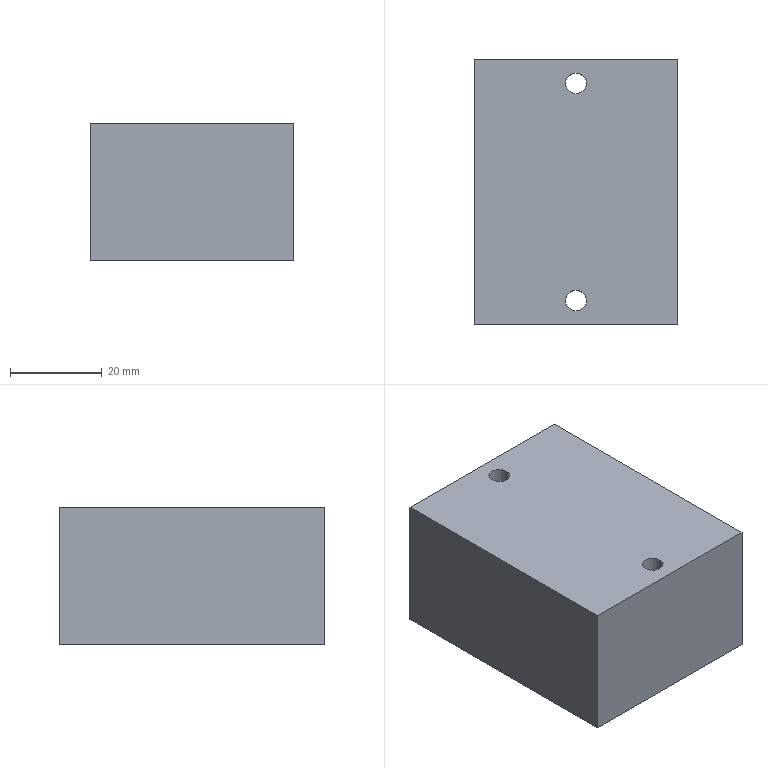Part | SolidWorks | features Extrusion 1 | 1 solid | 10 faces | box 44.5 x 58 x 30 mm | volume 76476 mm3 | plane 6 | cylinder 4 | commonest cylinder face diameters 4.5 x4
STEP:
#1=CARTESIAN_POINT('',(-2.25,-23.7,30.));
#2=VERTEX_POINT('',#1);
#3=CARTESIAN_POINT('',(2.25,-23.7,30.));
#4=VERTEX_POINT('',#3);
#5=CARTESIAN_POINT('',(0.,-23.7,30.));
#6=DIRECTION('',(0.,0.,1.));
#7=DIRECTION('',(1.,0.,0.));
#8=AXIS2_PLACEMENT_3D('',#5,#6,#7);
#9=CIRCLE('',#8,2.25);
#10=EDGE_CURVE('',#2,#4,#9,.T.);
#11=ORIENTED_EDGE('',*,*,#10,.T.);
#12=CARTESIAN_POINT('',(2.25,-23.7,0.));
#13=VERTEX_POINT('',#12);
#14=CARTESIAN_POINT('',(2.25,-23.7,30.));
#15=DIRECTION('',(0.,0.,-1.));
#16=VECTOR('',#15,1000.);
#17=LINE('',#14,#16);
#18=EDGE_CURVE('',#4,#13,#17,.T.);
#19=ORIENTED_EDGE('',*,*,#18,.T.);
#20=CARTESIAN_POINT('',(-2.25,-23.7,0.));
#21=VERTEX_POINT('',#20);
#22=CARTESIAN_POINT('',(0.,-23.7,0.));
#23=DIRECTION('',(0.,0.,1.));
#24=DIRECTION('',(1.,0.,0.));
#25=AXIS2_PLACEMENT_3D('',#22,#23,#24);
#26=CIRCLE('',#25,2.25);
#27=EDGE_CURVE('',#21,#13,#26,.T.);
#28=ORIENTED_EDGE('',*,*,#27,.F.);
#29=CARTESIAN_POINT('',(-2.25,-23.7,30.));
#30=DIRECTION('',(0.,0.,-1.));
#31=VECTOR('',#30,1000.);
#32=LINE('',#29,#31);
#33=EDGE_CURVE('',#2,#21,#32,.T.);
#34=ORIENTED_EDGE('',*,*,#33,.F.);
#35=EDGE_LOOP('',(#11,#19,#28,#34));
#36=FACE_OUTER_BOUND('',#35,.T.);
#37=CARTESIAN_POINT('',(0.,-23.7,30.));
#38=DIRECTION('',(0.,0.,-1.));
#39=DIRECTION('',(-1.,0.,0.));
#40=AXIS2_PLACEMENT_3D('',#37,#38,#39);
#41=CYLINDRICAL_SURFACE('',#40,2.25);
#42=ADVANCED_FACE('',(#36),#41,.F.);
#43=CARTESIAN_POINT('',(-2.25,23.7,30.));
#44=VERTEX_POINT('',#43);
#45=CARTESIAN_POINT('',(2.25,23.7,30.));
#46=VERTEX_POINT('',#45);
#47=CARTESIAN_POINT('',(0.,23.7,30.));
#48=DIRECTION('',(0.,0.,1.));
#49=DIRECTION('',(1.,0.,0.));
#50=AXIS2_PLACEMENT_3D('',#47,#48,#49);
#51=CIRCLE('',#50,2.25);
#52=EDGE_CURVE('',#44,#46,#51,.T.);
#53=ORIENTED_EDGE('',*,*,#52,.T.);
#54=CARTESIAN_POINT('',(2.25,23.7,0.));
#55=VERTEX_POINT('',#54);
#56=CARTESIAN_POINT('',(2.25,23.7,30.));
#57=DIRECTION('',(0.,0.,-1.));
#58=VECTOR('',#57,1000.);
#59=LINE('',#56,#58);
#60=EDGE_CURVE('',#46,#55,#59,.T.);
#61=ORIENTED_EDGE('',*,*,#60,.T.);
#62=CARTESIAN_POINT('',(-2.25,23.7,0.));
#63=VERTEX_POINT('',#62);
#64=CARTESIAN_POINT('',(0.,23.7,0.));
#65=DIRECTION('',(0.,0.,1.));
#66=DIRECTION('',(1.,0.,0.));
#67=AXIS2_PLACEMENT_3D('',#64,#65,#66);
#68=CIRCLE('',#67,2.25);
#69=EDGE_CURVE('',#63,#55,#68,.T.);
#70=ORIENTED_EDGE('',*,*,#69,.F.);
#71=CARTESIAN_POINT('',(-2.25,23.7,30.));
#72=DIRECTION('',(0.,0.,-1.));
#73=VECTOR('',#72,1000.);
#74=LINE('',#71,#73);
#75=EDGE_CURVE('',#44,#63,#74,.T.);
#76=ORIENTED_EDGE('',*,*,#75,.F.);
#77=EDGE_LOOP('',(#53,#61,#70,#76));
#78=FACE_OUTER_BOUND('',#77,.T.);
#79=CARTESIAN_POINT('',(0.,23.7,30.));
#80=DIRECTION('',(0.,0.,-1.));
#81=DIRECTION('',(-1.,0.,0.));
#82=AXIS2_PLACEMENT_3D('',#79,#80,#81);
#83=CYLINDRICAL_SURFACE('',#82,2.25);
#84=ADVANCED_FACE('',(#78),#83,.F.);
#85=CARTESIAN_POINT('',(22.25,-29.,30.));
#86=VERTEX_POINT('',#85);
#87=CARTESIAN_POINT('',(22.25,29.,30.));
#88=VERTEX_POINT('',#87);
#89=CARTESIAN_POINT('',(22.25,-29.,30.));
#90=DIRECTION('',(0.,1.,0.));
#91=VECTOR('',#90,1000.);
#92=LINE('',#89,#91);
#93=EDGE_CURVE('',#86,#88,#92,.T.);
#94=ORIENTED_EDGE('',*,*,#93,.T.);
#95=CARTESIAN_POINT('',(-22.25,29.,30.));
#96=VERTEX_POINT('',#95);
#97=CARTESIAN_POINT('',(-22.25,29.,30.));
#98=DIRECTION('',(-1.,0.,0.));
#99=VECTOR('',#98,1000.);
#100=LINE('',#97,#99);
#101=EDGE_CURVE('',#88,#96,#100,.T.);
#102=ORIENTED_EDGE('',*,*,#101,.T.);
#103=CARTESIAN_POINT('',(-22.25,-29.,30.));
#104=VERTEX_POINT('',#103);
#105=CARTESIAN_POINT('',(-22.25,-29.,30.));
#106=DIRECTION('',(0.,-1.,0.));
#107=VECTOR('',#106,1000.);
#108=LINE('',#105,#107);
#109=EDGE_CURVE('',#96,#104,#108,.T.);
#110=ORIENTED_EDGE('',*,*,#109,.T.);
#111=CARTESIAN_POINT('',(-22.25,-29.,30.));
#112=DIRECTION('',(1.,0.,0.));
#113=VECTOR('',#112,1000.);
#114=LINE('',#111,#113);
#115=EDGE_CURVE('',#104,#86,#114,.T.);
#116=ORIENTED_EDGE('',*,*,#115,.T.);
#117=EDGE_LOOP('',(#94,#102,#110,#116));
#118=FACE_OUTER_BOUND('',#117,.T.);
#119=ORIENTED_EDGE('',*,*,#52,.F.);
#120=CARTESIAN_POINT('',(0.,23.7,30.));
#121=DIRECTION('',(0.,0.,1.));
#122=DIRECTION('',(1.,0.,0.));
#123=AXIS2_PLACEMENT_3D('',#120,#121,#122);
#124=CIRCLE('',#123,2.25);
#125=EDGE_CURVE('',#46,#44,#124,.T.);
#126=ORIENTED_EDGE('',*,*,#125,.F.);
#127=EDGE_LOOP('',(#119,#126));
#128=FACE_BOUND('',#127,.T.);
#129=ORIENTED_EDGE('',*,*,#10,.F.);
#130=CARTESIAN_POINT('',(0.,-23.7,30.));
#131=DIRECTION('',(0.,0.,1.));
#132=DIRECTION('',(1.,0.,0.));
#133=AXIS2_PLACEMENT_3D('',#130,#131,#132);
#134=CIRCLE('',#133,2.25);
#135=EDGE_CURVE('',#4,#2,#134,.T.);
#136=ORIENTED_EDGE('',*,*,#135,.F.);
#137=EDGE_LOOP('',(#129,#136));
#138=FACE_BOUND('',#137,.T.);
#139=CARTESIAN_POINT('',(0.,0.,30.));
#140=DIRECTION('',(0.,0.,-1.));
#141=DIRECTION('',(-1.,0.,0.));
#142=AXIS2_PLACEMENT_3D('',#139,#140,#141);
#143=PLANE('',#142);
#144=ADVANCED_FACE('',(#118,#128,#138),#143,.F.);
#145=ORIENTED_EDGE('',*,*,#69,.T.);
#146=CARTESIAN_POINT('',(0.,23.7,0.));
#147=DIRECTION('',(0.,0.,1.));
#148=DIRECTION('',(1.,0.,0.));
#149=AXIS2_PLACEMENT_3D('',#146,#147,#148);
#150=CIRCLE('',#149,2.25);
#151=EDGE_CURVE('',#55,#63,#150,.T.);
#152=ORIENTED_EDGE('',*,*,#151,.T.);
#153=EDGE_LOOP('',(#145,#152));
#154=FACE_BOUND('',#153,.T.);
#155=CARTESIAN_POINT('',(22.25,-29.,0.));
#156=VERTEX_POINT('',#155);
#157=CARTESIAN_POINT('',(22.25,29.,0.));
#158=VERTEX_POINT('',#157);
#159=CARTESIAN_POINT('',(22.25,-29.,0.));
#160=DIRECTION('',(0.,1.,0.));
#161=VECTOR('',#160,1000.);
#162=LINE('',#159,#161);
#163=EDGE_CURVE('',#156,#158,#162,.T.);
#164=ORIENTED_EDGE('',*,*,#163,.F.);
#165=CARTESIAN_POINT('',(-22.25,-29.,0.));
#166=VERTEX_POINT('',#165);
#167=CARTESIAN_POINT('',(-22.25,-29.,0.));
#168=DIRECTION('',(1.,0.,0.));
#169=VECTOR('',#168,1000.);
#170=LINE('',#167,#169);
#171=EDGE_CURVE('',#166,#156,#170,.T.);
#172=ORIENTED_EDGE('',*,*,#171,.F.);
#173=CARTESIAN_POINT('',(-22.25,29.,0.));
#174=VERTEX_POINT('',#173);
#175=CARTESIAN_POINT('',(-22.25,-29.,0.));
#176=DIRECTION('',(0.,-1.,0.));
#177=VECTOR('',#176,1000.);
#178=LINE('',#175,#177);
#179=EDGE_CURVE('',#174,#166,#178,.T.);
#180=ORIENTED_EDGE('',*,*,#179,.F.);
#181=CARTESIAN_POINT('',(-22.25,29.,0.));
#182=DIRECTION('',(-1.,0.,0.));
#183=VECTOR('',#182,1000.);
#184=LINE('',#181,#183);
#185=EDGE_CURVE('',#158,#174,#184,.T.);
#186=ORIENTED_EDGE('',*,*,#185,.F.);
#187=EDGE_LOOP('',(#164,#172,#180,#186));
#188=FACE_OUTER_BOUND('',#187,.T.);
#189=ORIENTED_EDGE('',*,*,#27,.T.);
#190=CARTESIAN_POINT('',(0.,-23.7,0.));
#191=DIRECTION('',(0.,0.,1.));
#192=DIRECTION('',(1.,0.,0.));
#193=AXIS2_PLACEMENT_3D('',#190,#191,#192);
#194=CIRCLE('',#193,2.25);
#195=EDGE_CURVE('',#13,#21,#194,.T.);
#196=ORIENTED_EDGE('',*,*,#195,.T.);
#197=EDGE_LOOP('',(#189,#196));
#198=FACE_BOUND('',#197,.T.);
#199=CARTESIAN_POINT('',(0.,0.,0.));
#200=DIRECTION('',(0.,0.,-1.));
#201=DIRECTION('',(-1.,0.,0.));
#202=AXIS2_PLACEMENT_3D('',#199,#200,#201);
#203=PLANE('',#202);
#204=ADVANCED_FACE('',(#154,#188,#198),#203,.T.);
#205=ORIENTED_EDGE('',*,*,#163,.T.);
#206=CARTESIAN_POINT('',(22.25,29.,30.));
#207=DIRECTION('',(0.,0.,-1.));
#208=VECTOR('',#207,1000.);
#209=LINE('',#206,#208);
#210=EDGE_CURVE('',#88,#158,#209,.T.);
#211=ORIENTED_EDGE('',*,*,#210,.F.);
#212=ORIENTED_EDGE('',*,*,#93,.F.);
#213=CARTESIAN_POINT('',(22.25,-29.,30.));
#214=DIRECTION('',(0.,0.,-1.));
#215=VECTOR('',#214,1000.);
#216=LINE('',#213,#215);
#217=EDGE_CURVE('',#86,#156,#216,.T.);
#218=ORIENTED_EDGE('',*,*,#217,.T.);
#219=EDGE_LOOP('',(#205,#211,#212,#218));
#220=FACE_OUTER_BOUND('',#219,.T.);
#221=CARTESIAN_POINT('',(22.25,-29.,30.));
#222=DIRECTION('',(-1.,0.,0.));
#223=DIRECTION('',(0.,0.,1.));
#224=AXIS2_PLACEMENT_3D('',#221,#222,#223);
#225=PLANE('',#224);
#226=ADVANCED_FACE('',(#220),#225,.F.);
#227=ORIENTED_EDGE('',*,*,#185,.T.);
#228=CARTESIAN_POINT('',(-22.25,29.,30.));
#229=DIRECTION('',(0.,0.,-1.));
#230=VECTOR('',#229,1000.);
#231=LINE('',#228,#230);
#232=EDGE_CURVE('',#96,#174,#231,.T.);
#233=ORIENTED_EDGE('',*,*,#232,.F.);
#234=ORIENTED_EDGE('',*,*,#101,.F.);
#235=ORIENTED_EDGE('',*,*,#210,.T.);
#236=EDGE_LOOP('',(#227,#233,#234,#235));
#237=FACE_OUTER_BOUND('',#236,.T.);
#238=CARTESIAN_POINT('',(-22.25,29.,30.));
#239=DIRECTION('',(0.,-1.,0.));
#240=DIRECTION('',(0.,0.,-1.));
#241=AXIS2_PLACEMENT_3D('',#238,#239,#240);
#242=PLANE('',#241);
#243=ADVANCED_FACE('',(#237),#242,.F.);
#244=ORIENTED_EDGE('',*,*,#179,.T.);
#245=CARTESIAN_POINT('',(-22.25,-29.,30.));
#246=DIRECTION('',(0.,0.,-1.));
#247=VECTOR('',#246,1000.);
#248=LINE('',#245,#247);
#249=EDGE_CURVE('',#104,#166,#248,.T.);
#250=ORIENTED_EDGE('',*,*,#249,.F.);
#251=ORIENTED_EDGE('',*,*,#109,.F.);
#252=ORIENTED_EDGE('',*,*,#232,.T.);
#253=EDGE_LOOP('',(#244,#250,#251,#252));
#254=FACE_OUTER_BOUND('',#253,.T.);
#255=CARTESIAN_POINT('',(-22.25,-29.,30.));
#256=DIRECTION('',(1.,0.,0.));
#257=DIRECTION('',(0.,0.,-1.));
#258=AXIS2_PLACEMENT_3D('',#255,#256,#257);
#259=PLANE('',#258);
#260=ADVANCED_FACE('',(#254),#259,.F.);
#261=ORIENTED_EDGE('',*,*,#171,.T.);
#262=ORIENTED_EDGE('',*,*,#217,.F.);
#263=ORIENTED_EDGE('',*,*,#115,.F.);
#264=ORIENTED_EDGE('',*,*,#249,.T.);
#265=EDGE_LOOP('',(#261,#262,#263,#264));
#266=FACE_OUTER_BOUND('',#265,.T.);
#267=CARTESIAN_POINT('',(-22.25,-29.,30.));
#268=DIRECTION('',(0.,1.,0.));
#269=DIRECTION('',(0.,0.,1.));
#270=AXIS2_PLACEMENT_3D('',#267,#268,#269);
#271=PLANE('',#270);
#272=ADVANCED_FACE('',(#266),#271,.F.);
#273=ORIENTED_EDGE('',*,*,#60,.F.);
#274=ORIENTED_EDGE('',*,*,#125,.T.);
#275=ORIENTED_EDGE('',*,*,#75,.T.);
#276=ORIENTED_EDGE('',*,*,#151,.F.);
#277=EDGE_LOOP('',(#273,#274,#275,#276));
#278=FACE_OUTER_BOUND('',#277,.T.);
#279=CARTESIAN_POINT('',(0.,23.7,30.));
#280=DIRECTION('',(0.,0.,-1.));
#281=DIRECTION('',(-1.,0.,0.));
#282=AXIS2_PLACEMENT_3D('',#279,#280,#281);
#283=CYLINDRICAL_SURFACE('',#282,2.25);
#284=ADVANCED_FACE('',(#278),#283,.F.);
#285=ORIENTED_EDGE('',*,*,#18,.F.);
#286=ORIENTED_EDGE('',*,*,#135,.T.);
#287=ORIENTED_EDGE('',*,*,#33,.T.);
#288=ORIENTED_EDGE('',*,*,#195,.F.);
#289=EDGE_LOOP('',(#285,#286,#287,#288));
#290=FACE_OUTER_BOUND('',#289,.T.);
#291=CARTESIAN_POINT('',(0.,-23.7,30.));
#292=DIRECTION('',(0.,0.,-1.));
#293=DIRECTION('',(-1.,0.,0.));
#294=AXIS2_PLACEMENT_3D('',#291,#292,#293);
#295=CYLINDRICAL_SURFACE('',#294,2.25);
#296=ADVANCED_FACE('',(#290),#295,.F.);
#297=CLOSED_SHELL('',(#42,#84,#144,#204,#226,#243,#260,#272,#284,#296));
#298=MANIFOLD_SOLID_BREP('',#297);
#299=CARTESIAN_POINT('',(0.,0.,0.));
#300=DIRECTION('',(0.,0.,1.));
#301=DIRECTION('',(1.,0.,0.));
#302=AXIS2_PLACEMENT_3D('',#299,#300,#301);
#303=(LENGTH_UNIT()NAMED_UNIT(*)SI_UNIT(.MILLI.,.METRE.));
#304=UNCERTAINTY_MEASURE_WITH_UNIT(LENGTH_MEASURE(0.00001),#303,'','');
#305=(NAMED_UNIT(*)PLANE_ANGLE_UNIT()SI_UNIT($,.RADIAN.));
#306=(NAMED_UNIT(*)SI_UNIT($,.STERADIAN.)SOLID_ANGLE_UNIT());
#307=(GEOMETRIC_REPRESENTATION_CONTEXT(3)GLOBAL_UNCERTAINTY_ASSIGNED_CONTEXT((#304))GLOBAL_UNIT_ASSIGNED_CONTEXT((#303,#305,#306))REPRESENTATION_CONTEXT('',''));
#308=ADVANCED_BREP_SHAPE_REPRESENTATION('',(#298,#302),#307);